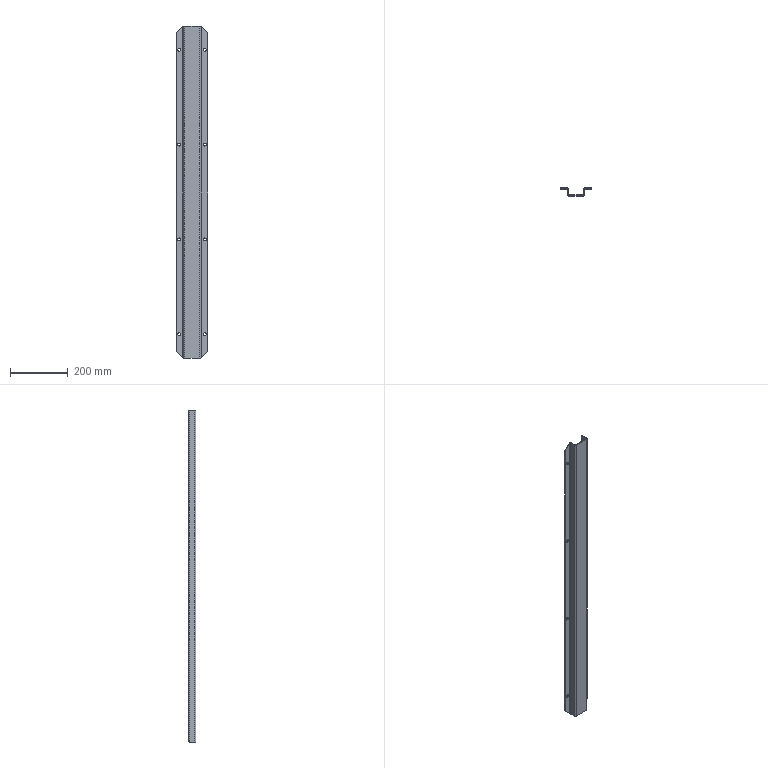Part | STEP file | 750038193 | 1 solid | 46 faces | box 108 x 27.5 x 1154 mm | volume 435104 mm3 | cylinder 24 | plane 18 | spline 4 | commonest cylinder face diameters 10.5 x16 4 x4 9 x4